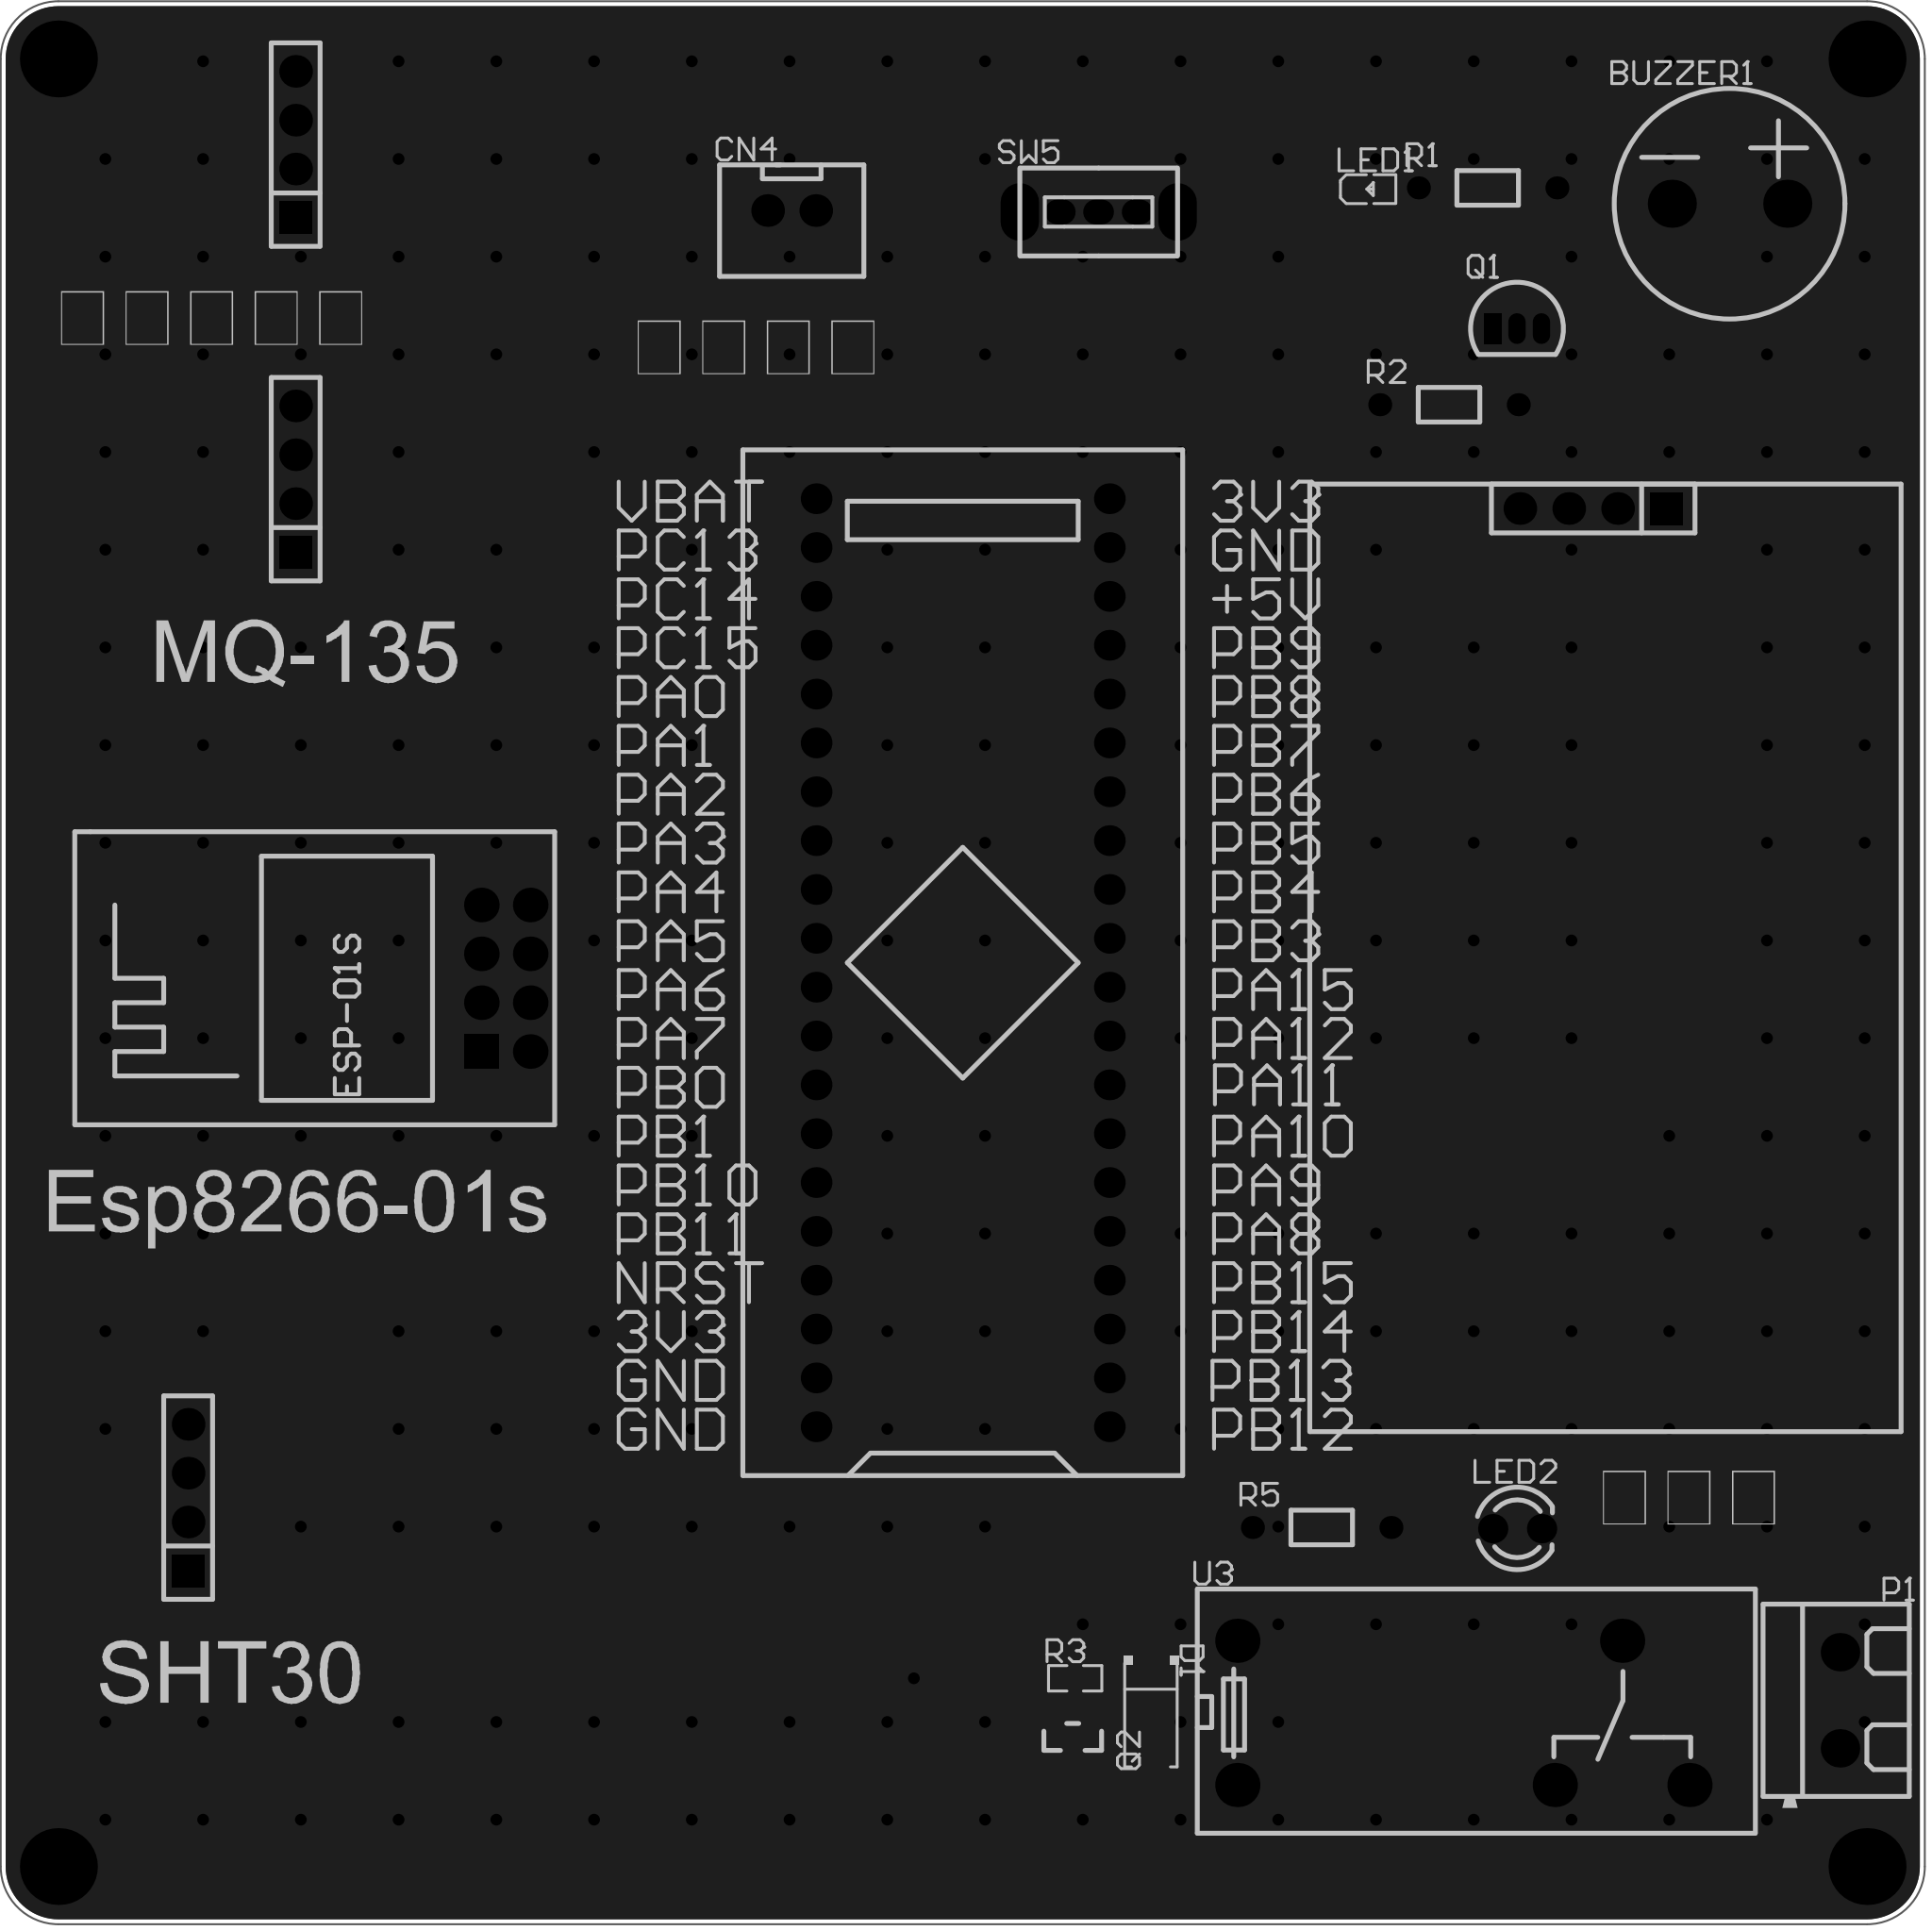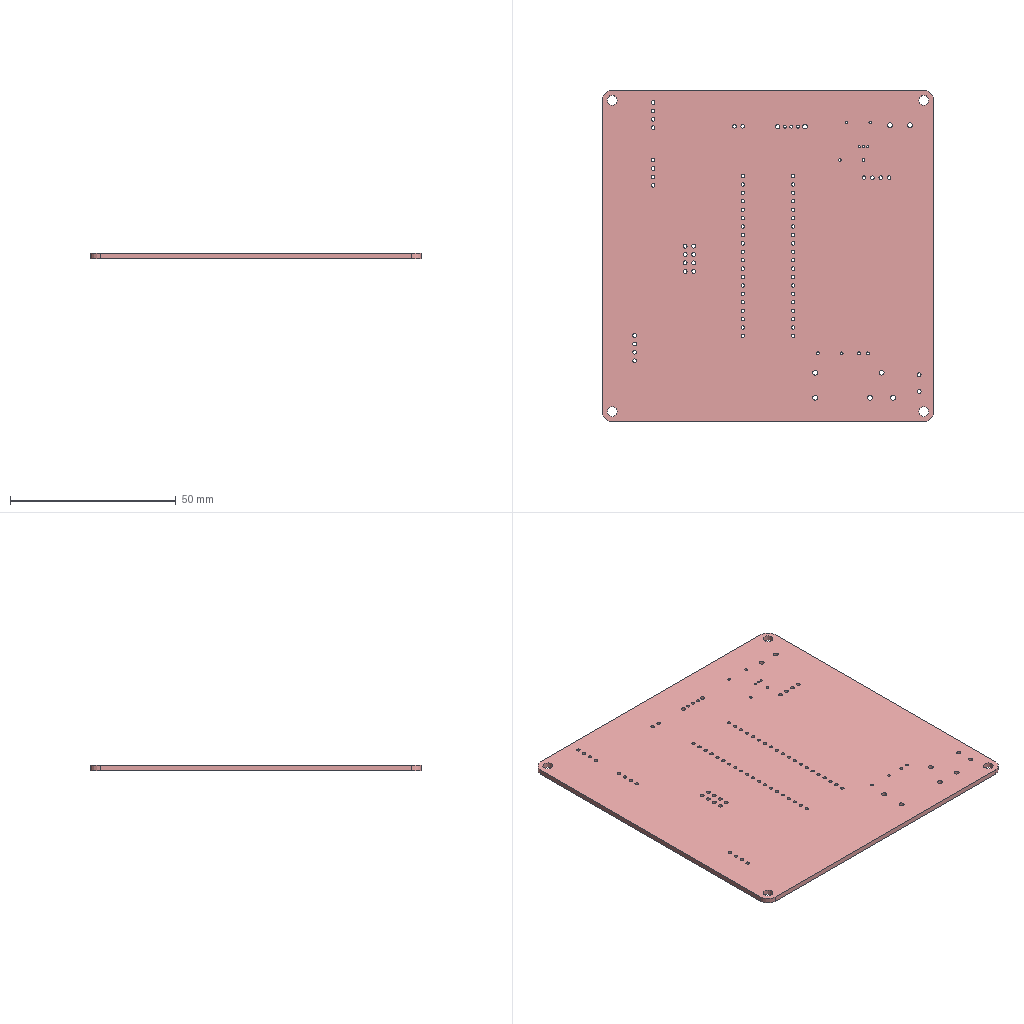Circuit board layout | Altium Designer | box 100 x 100 x 1.6 mm
Layer stack:
# Altium Designer layer stack of  (unit mm; dielectric type: 0 none, 1 core, 2 prepreg, 3 surface material)
index,name,kind,layer,copper_thickness_mm,dielectric_type,dielectric_thickness_mm,dielectric_material,dielectric_constant
0,Top Paste Mask Layer,other,,,,,,
1,Top Silkscreen Layer,other,,,,,,
2,Top Solder Mask Layer,dielectric,,,3,0.01,,3.3
3,Top Layer,copper,Top Layer,0.035,,,,
4,Dielectric1,dielectric,,,3,1.51,FR4,4.5
5,Bottom Layer,copper,Bottom Layer,0.035,,,,
6,Bottom Solder Mask Layer,dielectric,,,3,0.01,,3.3
7,Bottom Silkscreen Layer,other,,,,,,
8,Bottom Paste Mask Layer,other,,,,,,
# drill layer pairs: low layer,high layer
drill_pair,Top Layer,Bottom Layer
Part placement:
Designator,Comment,Layer,Footprint,Center-X(mm),Center-Y(mm),Rotation
U1,STM32F103C8T6-Card,TopLayer,CONN-TH_L53.3-W22.9_STM32F103C8T6-CARD,141.351,130.937,90
U2,ESP-01S,TopLayer,WIFIM-TH_ESP-01S,117.602,130.13,90
CN4,XH2.54*2P_直插,TopLayer,CONN-TH_2P-P2.50-XH2.54-2P,132.461,170.053,0
SW5,,TopLayer,拨动开关,148.417,169.978,0
H2,,TopLayer,HDR-TH_4P-P2.54-V-F,174.117,154.559,180
H4,,TopLayer,HDR-TH_4P-P2.54-V-F,106.68,156.083,90
H6,,TopLayer,HDR-TH_4P-P2.54-V-F,101.092,103.124,90
H1,,TopLayer,HDR-TH_4P-P2.54-V-F,106.68,173.482,90
BUZZER1,buzzer,TopLayer,BUZ-TH_BD12.0-P6.00-D0.9-RD,181.205,170.407,0
D1,,TopLayer,SMA_1N4007,151.13,91.821,270
LED1,,TopLayer,LED_0603,162.47,171.161,0
LED2,,TopLayer,LED_TH-3mm,170.167,101.507,0
P1,KF301-2P接线端子,TopLayer,CONN-TH_XY301V-A-5.0-2P,186.944,92.583,270
Q1,,TopLayer,S8050_TO_92,170.156,163.915,0
Q2,,TopLayer,S8050_SOT-23,147.066,90.678,90
R1,220Ω,TopLayer,Res_1/8W,168.633,171.232,0
R2,10kΩ,TopLayer,Res_1/8W,166.624,159.956,0
R3,1K,TopLayer,R0603,147.193,93.726,0
R5,1kΩ,TopLayer,Res_1/8W,160.007,101.569,0
U3,SSKD6132,TopLayer,RELAY-TH_G2R-1,167.373,91.927,0
Pad and via stacks:
# Altium Designer via and pad stacks of  (unit mm). Each distinct definition once, with the count of objects using it.
# via: kind,start_layer,end_layer,hole_mm,diameter_mm,mode(0 simple;1 top-mid-bottom;2 full stack),diameter_per_layer,count,example_net
# pad: kind,layer,hole_mm,hole_type(0 round;1 square;2 slot),plating,top_size,top_shape(1 round;2 rect;3 octagon;9 rounded rect),mid_size,bottom_size,mode,footprint,size_per_layer,count,example
pad,Multi-Layer,3,0,plated,4x4,1,4x4,4x4,0,,,4,1
pad,Multi-Layer,1,0,plated,1.6x1.6,1,1.6x1.6,1.6x1.6,0,CONN-TH_L53.3-W22.9_STM32F103C8T6-CARD,,40,U1.1
pad,Multi-Layer,1.2,0,plated,1.8x1.8,2,1.8x1.8,1.8x1.8,0,WIFIM-TH_ESP-01S,,1,U2.1
pad,Multi-Layer,1.2,0,plated,1.8x1.8,1,1.8x1.8,1.8x1.8,0,WIFIM-TH_ESP-01S,,7,U2.2
pad,Multi-Layer,1.05,0,plated,1.7x1.7,1,1.7x1.7,1.7x1.7,0,CONN-TH_2P-P2.50-XH2.54-2P,,2,CN4.2
pad,Multi-Layer,0.8992,0,plated,1.6x1.3,1,1.6x1.3,1.6x1.3,0,\u00B2\u00A6\u00B6\u00AF\u00BF\u00AA\u00B9\u00D8,,3,SW5.1
pad,Multi-Layer,1.3,0,plated,3x1.999,1,3x1.999,3x1.999,0,\u00B2\u00A6\u00B6\u00AF\u00BF\u00AA\u00B9\u00D8,,2,SW5.4
pad,Multi-Layer,1.1,0,plated,1.7x1.7,2,1.7x1.7,1.7x1.7,0,HDR-TH_4P-P2.54-V-F,,4,H2.1
pad,Multi-Layer,1.1,0,plated,1.7x1.7,1,1.7x1.7,1.7x1.7,0,HDR-TH_4P-P2.54-V-F,,12,H2.2
pad,Multi-Layer,1.5,0,plated,2.5x2.5,1,2.5x2.5,2.5x2.5,0,BUZ-TH_BD12.0-P6.00-D0.9-RD,,2,BUZZER1.1
pad,Multi-Layer,0.9144,0,plated,1.524x1.524,1,1.524x1.524,1.524x1.524,0,LED_TH-3mm,,2,LED2.1
pad,Multi-Layer,1.2,0,plated,2x2,1,2x2,2x2,0,CONN-TH_XY301V-A-5.0-2P,,2,P1.1
pad,Multi-Layer,0.701,0,plated,0.8992x1.6,2,0.8992x1.6,0.8992x1.6,0,S8050_TO_92,,1,Q1.1
pad,Multi-Layer,0.701,0,plated,0.8992x1.6,1,0.8992x1.6,0.8992x1.6,0,S8050_TO_92,,2,Q1.2
pad,Multi-Layer,0.8001,0,plated,1.199x1.199,1,1.199x1.199,1.199x1.199,0,Res_1/8W,,6,R1.1
pad,Multi-Layer,1.5,0,plated,2.3x2.3,1,2.3x2.3,2.3x2.3,0,RELAY-TH_G2R-1,,5,U3.3
pad,Top Layer,0,0,plated,2.046x1.62,2,2.046x1.62,2.046x1.62,0,SMA_1N4007,,2,D1.2
pad,Top Layer,0,0,plated,0.8001x0.8001,2,0.8001x0.8001,0.8001x0.8001,0,LED_0603,,2,LED1.1
pad,Top Layer,0,0,plated,1x0.8,2,1x0.8,1x0.8,0,S8050_SOT-23,,3,Q2.2
pad,Top Layer,0,0,plated,0.8065x0.864,2,0.8065x0.864,0.8065x0.864,0,R0603,,2,R3.2
via,Top Layer,Bottom Layer,0.3048,0.61,0,,278,PB1
Copper pours:
name,layer,net,type(0 solid;1 hatched;2 none)
Bottom Layer-GND,Bottom Layer,GND,0
Top Layer-GND,Top Layer,GND,0